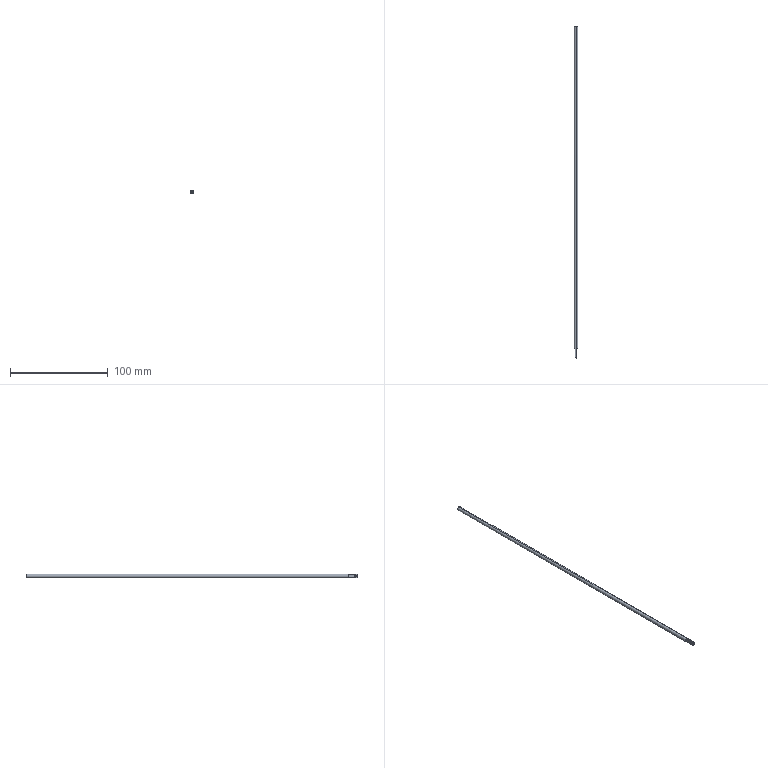Part | SolidWorks | features ICE 2, Extrusion 1, Fillet 1 | 1 solid | 14 faces | box 4 x 340 x 4 mm | volume 4216 mm3 | plane 6 | torus 4 | cylinder 4 | commonest cylinder face diameters 2 x2 4 x2
STEP:
#1=CARTESIAN_POINT('',(0.,-339.,2.));
#2=VERTEX_POINT('',#1);
#3=CARTESIAN_POINT('',(1.,-339.,1.732));
#4=VERTEX_POINT('',#3);
#5=CARTESIAN_POINT('',(0.,-339.,0.));
#6=DIRECTION('',(0.,1.,0.));
#7=DIRECTION('',(0.,0.,-1.));
#8=AXIS2_PLACEMENT_3D('',#5,#6,#7);
#9=CIRCLE('',#8,2.);
#10=EDGE_CURVE('',#2,#4,#9,.T.);
#11=ORIENTED_EDGE('',*,*,#10,.F.);
#12=CARTESIAN_POINT('',(0.,-340.,1.));
#13=VERTEX_POINT('',#12);
#14=CARTESIAN_POINT('',(0.,-339.,1.));
#15=DIRECTION('',(1.,0.,0.));
#16=DIRECTION('',(0.,0.,-1.));
#17=AXIS2_PLACEMENT_3D('',#14,#15,#16);
#18=CIRCLE('',#17,1.);
#19=EDGE_CURVE('',#2,#13,#18,.T.);
#20=ORIENTED_EDGE('',*,*,#19,.T.);
#21=CARTESIAN_POINT('',(1.,-340.,0.));
#22=VERTEX_POINT('',#21);
#23=CARTESIAN_POINT('',(0.,-340.,0.));
#24=DIRECTION('',(0.,-1.,0.));
#25=DIRECTION('',(0.,0.,-1.));
#26=AXIS2_PLACEMENT_3D('',#23,#24,#25);
#27=CIRCLE('',#26,1.);
#28=EDGE_CURVE('',#22,#13,#27,.T.);
#29=ORIENTED_EDGE('',*,*,#28,.F.);
#30=CARTESIAN_POINT('',(1.,-339.,1.732));
#31=CARTESIAN_POINT('',(1.,-339.19,1.732));
#32=CARTESIAN_POINT('',(1.,-339.375,1.668));
#33=CARTESIAN_POINT('',(1.,-339.68,1.444));
#34=CARTESIAN_POINT('',(1.,-339.795,1.286));
#35=CARTESIAN_POINT('',(1.,-339.905,1.026));
#36=CARTESIAN_POINT('',(1.,-339.932,0.9344));
#37=CARTESIAN_POINT('',(1.,-339.971,0.7509));
#38=CARTESIAN_POINT('',(1.,-339.982,0.658));
#39=CARTESIAN_POINT('',(1.,-340.003,0.3774));
#40=CARTESIAN_POINT('',(1.,-340.,0.1883));
#41=CARTESIAN_POINT('',(1.,-340.,0.));
#42=B_SPLINE_CURVE_WITH_KNOTS('',3,(#30,#31,#32,#33,#34,#35,#36,#37,#38,#39,#40,#41),.UNSPECIFIED.,.F.,.F.,(4,2,2,2,2,4),(0.,0.0005629,0.001126,0.001407,0.001689,0.002251),.UNSPECIFIED.);
#43=EDGE_CURVE('',#4,#22,#42,.T.);
#44=ORIENTED_EDGE('',*,*,#43,.F.);
#45=EDGE_LOOP('',(#11,#20,#29,#44));
#46=FACE_OUTER_BOUND('',#45,.T.);
#47=CARTESIAN_POINT('',(0.,-339.,0.));
#48=DIRECTION('',(0.,-1.,0.));
#49=DIRECTION('',(0.,0.,-1.));
#50=AXIS2_PLACEMENT_3D('',#47,#48,#49);
#51=TOROIDAL_SURFACE('',#50,1.,1.);
#52=ADVANCED_FACE('',(#46),#51,.T.);
#53=CARTESIAN_POINT('',(0.,-339.,-2.));
#54=VERTEX_POINT('',#53);
#55=CARTESIAN_POINT('',(-1.,-339.,-1.732));
#56=VERTEX_POINT('',#55);
#57=CARTESIAN_POINT('',(0.,-339.,0.));
#58=DIRECTION('',(0.,1.,0.));
#59=DIRECTION('',(0.,0.,-1.));
#60=AXIS2_PLACEMENT_3D('',#57,#58,#59);
#61=CIRCLE('',#60,2.);
#62=EDGE_CURVE('',#54,#56,#61,.T.);
#63=ORIENTED_EDGE('',*,*,#62,.F.);
#64=CARTESIAN_POINT('',(0.,-340.,-1.));
#65=VERTEX_POINT('',#64);
#66=CARTESIAN_POINT('',(0.,-339.,-1.));
#67=DIRECTION('',(-1.,0.,0.));
#68=DIRECTION('',(0.,0.,1.));
#69=AXIS2_PLACEMENT_3D('',#66,#67,#68);
#70=CIRCLE('',#69,1.);
#71=EDGE_CURVE('',#54,#65,#70,.T.);
#72=ORIENTED_EDGE('',*,*,#71,.T.);
#73=CARTESIAN_POINT('',(-1.,-340.,0.));
#74=VERTEX_POINT('',#73);
#75=CARTESIAN_POINT('',(0.,-340.,0.));
#76=DIRECTION('',(0.,-1.,0.));
#77=DIRECTION('',(0.,0.,-1.));
#78=AXIS2_PLACEMENT_3D('',#75,#76,#77);
#79=CIRCLE('',#78,1.);
#80=EDGE_CURVE('',#74,#65,#79,.T.);
#81=ORIENTED_EDGE('',*,*,#80,.F.);
#82=CARTESIAN_POINT('',(-1.,-339.,-1.732));
#83=CARTESIAN_POINT('',(-1.,-339.19,-1.732));
#84=CARTESIAN_POINT('',(-1.,-339.375,-1.668));
#85=CARTESIAN_POINT('',(-1.,-339.68,-1.444));
#86=CARTESIAN_POINT('',(-1.,-339.795,-1.286));
#87=CARTESIAN_POINT('',(-1.,-339.905,-1.026));
#88=CARTESIAN_POINT('',(-1.,-339.932,-0.9344));
#89=CARTESIAN_POINT('',(-1.,-339.971,-0.7509));
#90=CARTESIAN_POINT('',(-1.,-339.982,-0.658));
#91=CARTESIAN_POINT('',(-1.,-340.003,-0.3774));
#92=CARTESIAN_POINT('',(-1.,-340.,-0.1883));
#93=CARTESIAN_POINT('',(-1.,-340.,0.));
#94=B_SPLINE_CURVE_WITH_KNOTS('',3,(#82,#83,#84,#85,#86,#87,#88,#89,#90,#91,#92,#93),.UNSPECIFIED.,.F.,.F.,(4,2,2,2,2,4),(0.,0.0005629,0.001126,0.001407,0.001689,0.002251),.UNSPECIFIED.);
#95=EDGE_CURVE('',#56,#74,#94,.T.);
#96=ORIENTED_EDGE('',*,*,#95,.F.);
#97=EDGE_LOOP('',(#63,#72,#81,#96));
#98=FACE_OUTER_BOUND('',#97,.T.);
#99=CARTESIAN_POINT('',(0.,-339.,0.));
#100=DIRECTION('',(0.,-1.,0.));
#101=DIRECTION('',(0.,0.,-1.));
#102=AXIS2_PLACEMENT_3D('',#99,#100,#101);
#103=TOROIDAL_SURFACE('',#102,1.,1.);
#104=ADVANCED_FACE('',(#98),#103,.T.);
#105=CARTESIAN_POINT('',(1.,-337.5,-1.));
#106=VERTEX_POINT('',#105);
#107=CARTESIAN_POINT('',(1.,-337.5,1.));
#108=VERTEX_POINT('',#107);
#109=CARTESIAN_POINT('',(1.,-337.5,0.));
#110=DIRECTION('',(-1.,0.,0.));
#111=DIRECTION('',(0.,-1.,0.));
#112=AXIS2_PLACEMENT_3D('',#109,#110,#111);
#113=CIRCLE('',#112,1.);
#114=EDGE_CURVE('',#106,#108,#113,.T.);
#115=ORIENTED_EDGE('',*,*,#114,.F.);
#116=CARTESIAN_POINT('',(-1.,-337.5,-1.));
#117=VERTEX_POINT('',#116);
#118=CARTESIAN_POINT('',(399.,-337.5,-1.));
#119=DIRECTION('',(-1.,0.,0.));
#120=VECTOR('',#119,1000.);
#121=LINE('',#118,#120);
#122=EDGE_CURVE('',#106,#117,#121,.T.);
#123=ORIENTED_EDGE('',*,*,#122,.T.);
#124=CARTESIAN_POINT('',(-1.,-337.5,1.));
#125=VERTEX_POINT('',#124);
#126=CARTESIAN_POINT('',(-1.,-337.5,0.));
#127=DIRECTION('',(-1.,0.,0.));
#128=DIRECTION('',(0.,0.,1.));
#129=AXIS2_PLACEMENT_3D('',#126,#127,#128);
#130=CIRCLE('',#129,1.);
#131=EDGE_CURVE('',#117,#125,#130,.T.);
#132=ORIENTED_EDGE('',*,*,#131,.T.);
#133=CARTESIAN_POINT('',(399.,-337.5,1.));
#134=DIRECTION('',(-1.,0.,0.));
#135=VECTOR('',#134,1000.);
#136=LINE('',#133,#135);
#137=EDGE_CURVE('',#108,#125,#136,.T.);
#138=ORIENTED_EDGE('',*,*,#137,.F.);
#139=EDGE_LOOP('',(#115,#123,#132,#138));
#140=FACE_OUTER_BOUND('',#139,.T.);
#141=CARTESIAN_POINT('',(399.,-337.5,0.));
#142=DIRECTION('',(-1.,0.,0.));
#143=DIRECTION('',(0.,0.,1.));
#144=AXIS2_PLACEMENT_3D('',#141,#142,#143);
#145=CYLINDRICAL_SURFACE('',#144,1.);
#146=ADVANCED_FACE('',(#140),#145,.F.);
#147=CARTESIAN_POINT('',(1.,-339.,-1.732));
#148=VERTEX_POINT('',#147);
#149=CARTESIAN_POINT('',(0.,-339.,0.));
#150=DIRECTION('',(0.,1.,0.));
#151=DIRECTION('',(0.,0.,-1.));
#152=AXIS2_PLACEMENT_3D('',#149,#150,#151);
#153=CIRCLE('',#152,2.);
#154=EDGE_CURVE('',#148,#54,#153,.T.);
#155=ORIENTED_EDGE('',*,*,#154,.T.);
#156=CARTESIAN_POINT('',(0.,0.,-2.));
#157=VERTEX_POINT('',#156);
#158=CARTESIAN_POINT('',(0.,-340.,-2.));
#159=DIRECTION('',(0.,1.,0.));
#160=VECTOR('',#159,1000.);
#161=LINE('',#158,#160);
#162=EDGE_CURVE('',#54,#157,#161,.T.);
#163=ORIENTED_EDGE('',*,*,#162,.T.);
#164=CARTESIAN_POINT('',(0.,0.,2.));
#165=VERTEX_POINT('',#164);
#166=CARTESIAN_POINT('',(0.,0.,0.));
#167=DIRECTION('',(0.,-1.,0.));
#168=DIRECTION('',(0.,0.,-1.));
#169=AXIS2_PLACEMENT_3D('',#166,#167,#168);
#170=CIRCLE('',#169,2.);
#171=EDGE_CURVE('',#157,#165,#170,.T.);
#172=ORIENTED_EDGE('',*,*,#171,.T.);
#173=CARTESIAN_POINT('',(0.,-340.,2.));
#174=DIRECTION('',(0.,1.,0.));
#175=VECTOR('',#174,1000.);
#176=LINE('',#173,#175);
#177=EDGE_CURVE('',#2,#165,#176,.T.);
#178=ORIENTED_EDGE('',*,*,#177,.F.);
#179=ORIENTED_EDGE('',*,*,#10,.T.);
#180=CARTESIAN_POINT('',(1.,-330.,1.732));
#181=VERTEX_POINT('',#180);
#182=CARTESIAN_POINT('',(1.,-340.,1.732));
#183=DIRECTION('',(0.,1.,0.));
#184=VECTOR('',#183,1000.);
#185=LINE('',#182,#184);
#186=EDGE_CURVE('',#4,#181,#185,.T.);
#187=ORIENTED_EDGE('',*,*,#186,.T.);
#188=CARTESIAN_POINT('',(1.,-330.,-1.732));
#189=VERTEX_POINT('',#188);
#190=CARTESIAN_POINT('',(0.,-330.,0.));
#191=DIRECTION('',(0.,1.,0.));
#192=DIRECTION('',(0.,0.,1.));
#193=AXIS2_PLACEMENT_3D('',#190,#191,#192);
#194=CIRCLE('',#193,2.);
#195=EDGE_CURVE('',#181,#189,#194,.T.);
#196=ORIENTED_EDGE('',*,*,#195,.T.);
#197=CARTESIAN_POINT('',(1.,-340.,-1.732));
#198=DIRECTION('',(0.,-1.,0.));
#199=VECTOR('',#198,1000.);
#200=LINE('',#197,#199);
#201=EDGE_CURVE('',#189,#148,#200,.T.);
#202=ORIENTED_EDGE('',*,*,#201,.T.);
#203=EDGE_LOOP('',(#155,#163,#172,#178,#179,#187,#196,#202));
#204=FACE_OUTER_BOUND('',#203,.T.);
#205=CARTESIAN_POINT('',(0.,-340.,0.));
#206=DIRECTION('',(0.,1.,0.));
#207=DIRECTION('',(0.,0.,1.));
#208=AXIS2_PLACEMENT_3D('',#205,#206,#207);
#209=CYLINDRICAL_SURFACE('',#208,2.);
#210=ADVANCED_FACE('',(#204),#209,.T.);
#211=ORIENTED_EDGE('',*,*,#162,.F.);
#212=ORIENTED_EDGE('',*,*,#62,.T.);
#213=CARTESIAN_POINT('',(-1.,-330.,-1.732));
#214=VERTEX_POINT('',#213);
#215=CARTESIAN_POINT('',(-1.,-340.,-1.732));
#216=DIRECTION('',(0.,1.,0.));
#217=VECTOR('',#216,1000.);
#218=LINE('',#215,#217);
#219=EDGE_CURVE('',#56,#214,#218,.T.);
#220=ORIENTED_EDGE('',*,*,#219,.T.);
#221=CARTESIAN_POINT('',(-1.,-330.,1.732));
#222=VERTEX_POINT('',#221);
#223=CARTESIAN_POINT('',(0.,-330.,0.));
#224=DIRECTION('',(0.,1.,0.));
#225=DIRECTION('',(0.,0.,1.));
#226=AXIS2_PLACEMENT_3D('',#223,#224,#225);
#227=CIRCLE('',#226,2.);
#228=EDGE_CURVE('',#214,#222,#227,.T.);
#229=ORIENTED_EDGE('',*,*,#228,.T.);
#230=CARTESIAN_POINT('',(-1.,-339.,1.732));
#231=VERTEX_POINT('',#230);
#232=CARTESIAN_POINT('',(-1.,-340.,1.732));
#233=DIRECTION('',(0.,-1.,0.));
#234=VECTOR('',#233,1000.);
#235=LINE('',#232,#234);
#236=EDGE_CURVE('',#222,#231,#235,.T.);
#237=ORIENTED_EDGE('',*,*,#236,.T.);
#238=CARTESIAN_POINT('',(0.,-339.,0.));
#239=DIRECTION('',(0.,1.,0.));
#240=DIRECTION('',(0.,0.,-1.));
#241=AXIS2_PLACEMENT_3D('',#238,#239,#240);
#242=CIRCLE('',#241,2.);
#243=EDGE_CURVE('',#231,#2,#242,.T.);
#244=ORIENTED_EDGE('',*,*,#243,.T.);
#245=ORIENTED_EDGE('',*,*,#177,.T.);
#246=CARTESIAN_POINT('',(0.,0.,0.));
#247=DIRECTION('',(0.,-1.,0.));
#248=DIRECTION('',(0.,0.,-1.));
#249=AXIS2_PLACEMENT_3D('',#246,#247,#248);
#250=CIRCLE('',#249,2.);
#251=EDGE_CURVE('',#165,#157,#250,.T.);
#252=ORIENTED_EDGE('',*,*,#251,.T.);
#253=EDGE_LOOP('',(#211,#212,#220,#229,#237,#244,#245,#252));
#254=FACE_OUTER_BOUND('',#253,.T.);
#255=CARTESIAN_POINT('',(0.,-340.,0.));
#256=DIRECTION('',(0.,1.,0.));
#257=DIRECTION('',(0.,0.,1.));
#258=AXIS2_PLACEMENT_3D('',#255,#256,#257);
#259=CYLINDRICAL_SURFACE('',#258,2.);
#260=ADVANCED_FACE('',(#254),#259,.T.);
#261=ORIENTED_EDGE('',*,*,#28,.T.);
#262=CARTESIAN_POINT('',(0.,-340.,0.));
#263=DIRECTION('',(0.,-1.,0.));
#264=DIRECTION('',(0.,0.,-1.));
#265=AXIS2_PLACEMENT_3D('',#262,#263,#264);
#266=CIRCLE('',#265,1.);
#267=EDGE_CURVE('',#13,#74,#266,.T.);
#268=ORIENTED_EDGE('',*,*,#267,.T.);
#269=ORIENTED_EDGE('',*,*,#80,.T.);
#270=CARTESIAN_POINT('',(0.,-340.,0.));
#271=DIRECTION('',(0.,-1.,0.));
#272=DIRECTION('',(0.,0.,-1.));
#273=AXIS2_PLACEMENT_3D('',#270,#271,#272);
#274=CIRCLE('',#273,1.);
#275=EDGE_CURVE('',#65,#22,#274,.T.);
#276=ORIENTED_EDGE('',*,*,#275,.T.);
#277=EDGE_LOOP('',(#261,#268,#269,#276));
#278=FACE_OUTER_BOUND('',#277,.T.);
#279=CARTESIAN_POINT('',(0.,-340.,0.));
#280=DIRECTION('',(0.,-1.,0.));
#281=DIRECTION('',(0.,0.,-1.));
#282=AXIS2_PLACEMENT_3D('',#279,#280,#281);
#283=PLANE('',#282);
#284=ADVANCED_FACE('',(#278),#283,.T.);
#285=ORIENTED_EDGE('',*,*,#251,.F.);
#286=ORIENTED_EDGE('',*,*,#171,.F.);
#287=EDGE_LOOP('',(#285,#286));
#288=FACE_OUTER_BOUND('',#287,.T.);
#289=CARTESIAN_POINT('',(0.,0.,0.));
#290=DIRECTION('',(0.,-1.,0.));
#291=DIRECTION('',(0.,0.,-1.));
#292=AXIS2_PLACEMENT_3D('',#289,#290,#291);
#293=PLANE('',#292);
#294=ADVANCED_FACE('',(#288),#293,.F.);
#295=CARTESIAN_POINT('',(1.,-330.,-200.));
#296=DIRECTION('',(0.,0.,1.));
#297=VECTOR('',#296,1000.);
#298=LINE('',#295,#297);
#299=EDGE_CURVE('',#189,#181,#298,.T.);
#300=ORIENTED_EDGE('',*,*,#299,.F.);
#301=ORIENTED_EDGE('',*,*,#195,.F.);
#302=EDGE_LOOP('',(#300,#301));
#303=FACE_OUTER_BOUND('',#302,.T.);
#304=CARTESIAN_POINT('',(1.,-330.,-200.));
#305=DIRECTION('',(0.,1.,0.));
#306=DIRECTION('',(0.,0.,1.));
#307=AXIS2_PLACEMENT_3D('',#304,#305,#306);
#308=PLANE('',#307);
#309=ADVANCED_FACE('',(#303),#308,.F.);
#310=CARTESIAN_POINT('',(1.,-337.5,0.));
#311=DIRECTION('',(-1.,0.,0.));
#312=DIRECTION('',(0.,-1.,0.));
#313=AXIS2_PLACEMENT_3D('',#310,#311,#312);
#314=CIRCLE('',#313,1.);
#315=EDGE_CURVE('',#108,#106,#314,.T.);
#316=ORIENTED_EDGE('',*,*,#315,.T.);
#317=ORIENTED_EDGE('',*,*,#114,.T.);
#318=EDGE_LOOP('',(#316,#317));
#319=FACE_BOUND('',#318,.T.);
#320=ORIENTED_EDGE('',*,*,#43,.T.);
#321=CARTESIAN_POINT('',(1.,-340.,0.));
#322=CARTESIAN_POINT('',(1.,-340.,-0.1868));
#323=CARTESIAN_POINT('',(1.,-340.003,-0.3739));
#324=CARTESIAN_POINT('',(1.,-339.983,-0.6523));
#325=CARTESIAN_POINT('',(1.,-339.972,-0.7447));
#326=CARTESIAN_POINT('',(1.,-339.934,-0.9281));
#327=CARTESIAN_POINT('',(1.,-339.907,-1.02));
#328=CARTESIAN_POINT('',(1.,-339.797,-1.282));
#329=CARTESIAN_POINT('',(1.,-339.684,-1.44));
#330=CARTESIAN_POINT('',(1.,-339.454,-1.611));
#331=CARTESIAN_POINT('',(1.,-339.37,-1.655));
#332=CARTESIAN_POINT('',(1.,-339.191,-1.716));
#333=CARTESIAN_POINT('',(1.,-339.096,-1.732));
#334=CARTESIAN_POINT('',(1.,-339.,-1.732));
#335=B_SPLINE_CURVE_WITH_KNOTS('',3,(#321,#322,#323,#324,#325,#326,#327,#328,#329,#330,#331,#332,#333,#334),.UNSPECIFIED.,.F.,.F.,(4,2,2,2,2,2,4),(0.,0.0005582,0.0008373,0.001116,0.001675,0.001954,0.002233),.UNSPECIFIED.);
#336=EDGE_CURVE('',#22,#148,#335,.T.);
#337=ORIENTED_EDGE('',*,*,#336,.T.);
#338=ORIENTED_EDGE('',*,*,#201,.F.);
#339=ORIENTED_EDGE('',*,*,#299,.T.);
#340=ORIENTED_EDGE('',*,*,#186,.F.);
#341=EDGE_LOOP('',(#320,#337,#338,#339,#340));
#342=FACE_OUTER_BOUND('',#341,.T.);
#343=CARTESIAN_POINT('',(1.,-340.,-200.));
#344=DIRECTION('',(-1.,0.,0.));
#345=DIRECTION('',(0.,-1.,0.));
#346=AXIS2_PLACEMENT_3D('',#343,#344,#345);
#347=PLANE('',#346);
#348=ADVANCED_FACE('',(#319,#342),#347,.F.);
#349=CARTESIAN_POINT('',(-1.,-330.,-200.));
#350=DIRECTION('',(0.,0.,1.));
#351=VECTOR('',#350,1000.);
#352=LINE('',#349,#351);
#353=EDGE_CURVE('',#214,#222,#352,.T.);
#354=ORIENTED_EDGE('',*,*,#353,.T.);
#355=ORIENTED_EDGE('',*,*,#228,.F.);
#356=EDGE_LOOP('',(#354,#355));
#357=FACE_OUTER_BOUND('',#356,.T.);
#358=CARTESIAN_POINT('',(-1.,-330.,-200.));
#359=DIRECTION('',(0.,1.,0.));
#360=DIRECTION('',(0.,0.,1.));
#361=AXIS2_PLACEMENT_3D('',#358,#359,#360);
#362=PLANE('',#361);
#363=ADVANCED_FACE('',(#357),#362,.F.);
#364=CARTESIAN_POINT('',(-1.,-337.5,0.));
#365=DIRECTION('',(-1.,0.,0.));
#366=DIRECTION('',(0.,0.,1.));
#367=AXIS2_PLACEMENT_3D('',#364,#365,#366);
#368=CIRCLE('',#367,1.);
#369=EDGE_CURVE('',#125,#117,#368,.T.);
#370=ORIENTED_EDGE('',*,*,#369,.F.);
#371=ORIENTED_EDGE('',*,*,#131,.F.);
#372=EDGE_LOOP('',(#370,#371));
#373=FACE_BOUND('',#372,.T.);
#374=ORIENTED_EDGE('',*,*,#219,.F.);
#375=ORIENTED_EDGE('',*,*,#95,.T.);
#376=CARTESIAN_POINT('',(-1.,-340.,0.));
#377=CARTESIAN_POINT('',(-1.,-340.,0.1868));
#378=CARTESIAN_POINT('',(-1.,-340.003,0.3739));
#379=CARTESIAN_POINT('',(-1.,-339.983,0.6523));
#380=CARTESIAN_POINT('',(-1.,-339.972,0.7447));
#381=CARTESIAN_POINT('',(-1.,-339.934,0.9281));
#382=CARTESIAN_POINT('',(-1.,-339.907,1.02));
#383=CARTESIAN_POINT('',(-1.,-339.797,1.282));
#384=CARTESIAN_POINT('',(-1.,-339.684,1.44));
#385=CARTESIAN_POINT('',(-1.,-339.454,1.611));
#386=CARTESIAN_POINT('',(-1.,-339.37,1.655));
#387=CARTESIAN_POINT('',(-1.,-339.191,1.716));
#388=CARTESIAN_POINT('',(-1.,-339.096,1.732));
#389=CARTESIAN_POINT('',(-1.,-339.,1.732));
#390=B_SPLINE_CURVE_WITH_KNOTS('',3,(#376,#377,#378,#379,#380,#381,#382,#383,#384,#385,#386,#387,#388,#389),.UNSPECIFIED.,.F.,.F.,(4,2,2,2,2,2,4),(0.,0.0005582,0.0008373,0.001116,0.001675,0.001954,0.002233),.UNSPECIFIED.);
#391=EDGE_CURVE('',#74,#231,#390,.T.);
#392=ORIENTED_EDGE('',*,*,#391,.T.);
#393=ORIENTED_EDGE('',*,*,#236,.F.);
#394=ORIENTED_EDGE('',*,*,#353,.F.);
#395=EDGE_LOOP('',(#374,#375,#392,#393,#394));
#396=FACE_OUTER_BOUND('',#395,.T.);
#397=CARTESIAN_POINT('',(-1.,-340.,-200.));
#398=DIRECTION('',(1.,0.,0.));
#399=DIRECTION('',(0.,1.,0.));
#400=AXIS2_PLACEMENT_3D('',#397,#398,#399);
#401=PLANE('',#400);
#402=ADVANCED_FACE('',(#373,#396),#401,.F.);
#403=ORIENTED_EDGE('',*,*,#122,.F.);
#404=ORIENTED_EDGE('',*,*,#315,.F.);
#405=ORIENTED_EDGE('',*,*,#137,.T.);
#406=ORIENTED_EDGE('',*,*,#369,.T.);
#407=EDGE_LOOP('',(#403,#404,#405,#406));
#408=FACE_OUTER_BOUND('',#407,.T.);
#409=CARTESIAN_POINT('',(399.,-337.5,0.));
#410=DIRECTION('',(-1.,0.,0.));
#411=DIRECTION('',(0.,0.,1.));
#412=AXIS2_PLACEMENT_3D('',#409,#410,#411);
#413=CYLINDRICAL_SURFACE('',#412,1.);
#414=ADVANCED_FACE('',(#408),#413,.F.);
#415=ORIENTED_EDGE('',*,*,#71,.F.);
#416=ORIENTED_EDGE('',*,*,#154,.F.);
#417=ORIENTED_EDGE('',*,*,#336,.F.);
#418=ORIENTED_EDGE('',*,*,#275,.F.);
#419=EDGE_LOOP('',(#415,#416,#417,#418));
#420=FACE_OUTER_BOUND('',#419,.T.);
#421=CARTESIAN_POINT('',(0.,-339.,0.));
#422=DIRECTION('',(0.,-1.,0.));
#423=DIRECTION('',(0.,0.,-1.));
#424=AXIS2_PLACEMENT_3D('',#421,#422,#423);
#425=TOROIDAL_SURFACE('',#424,1.,1.);
#426=ADVANCED_FACE('',(#420),#425,.T.);
#427=ORIENTED_EDGE('',*,*,#19,.F.);
#428=ORIENTED_EDGE('',*,*,#243,.F.);
#429=ORIENTED_EDGE('',*,*,#391,.F.);
#430=ORIENTED_EDGE('',*,*,#267,.F.);
#431=EDGE_LOOP('',(#427,#428,#429,#430));
#432=FACE_OUTER_BOUND('',#431,.T.);
#433=CARTESIAN_POINT('',(0.,-339.,0.));
#434=DIRECTION('',(0.,-1.,0.));
#435=DIRECTION('',(0.,0.,-1.));
#436=AXIS2_PLACEMENT_3D('',#433,#434,#435);
#437=TOROIDAL_SURFACE('',#436,1.,1.);
#438=ADVANCED_FACE('',(#432),#437,.T.);
#439=CLOSED_SHELL('',(#52,#104,#146,#210,#260,#284,#294,#309,#348,#363,#402,#414,#426,#438));
#440=MANIFOLD_SOLID_BREP('',#439);
#441=CARTESIAN_POINT('',(0.,0.,0.));
#442=DIRECTION('',(0.,0.,1.));
#443=DIRECTION('',(1.,0.,0.));
#444=AXIS2_PLACEMENT_3D('',#441,#442,#443);
#445=(LENGTH_UNIT()NAMED_UNIT(*)SI_UNIT(.MILLI.,.METRE.));
#446=UNCERTAINTY_MEASURE_WITH_UNIT(LENGTH_MEASURE(0.00001),#445,'','');
#447=(NAMED_UNIT(*)PLANE_ANGLE_UNIT()SI_UNIT($,.RADIAN.));
#448=(NAMED_UNIT(*)SI_UNIT($,.STERADIAN.)SOLID_ANGLE_UNIT());
#449=(GEOMETRIC_REPRESENTATION_CONTEXT(3)GLOBAL_UNCERTAINTY_ASSIGNED_CONTEXT((#446))GLOBAL_UNIT_ASSIGNED_CONTEXT((#445,#447,#448))REPRESENTATION_CONTEXT('',''));
#450=ADVANCED_BREP_SHAPE_REPRESENTATION('',(#440,#444),#449);